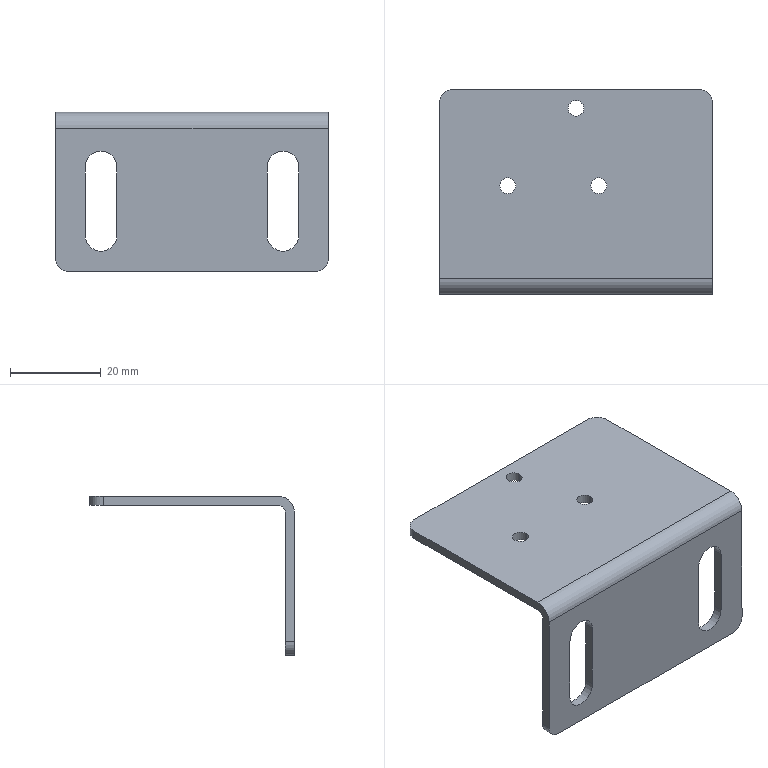Part | SolidWorks | features BaseBody 1 | 1 solid | 30 faces | box 60 x 45 x 35 mm | volume 8584 mm3 | cylinder 18 | plane 12 | commonest cylinder face diameters 7 x7 3.5 x6 6 x4 3 x1
STEP:
#1=CARTESIAN_POINT('',(-16.75,1.35,-2.));
#2=VERTEX_POINT('',#1);
#3=CARTESIAN_POINT('',(-13.25,1.35,-2.));
#4=VERTEX_POINT('',#3);
#5=CARTESIAN_POINT('',(-15.,1.35,-2.));
#6=DIRECTION('',(0.,0.,1.));
#7=DIRECTION('',(1.,0.,0.));
#8=AXIS2_PLACEMENT_3D('',#5,#6,#7);
#9=CIRCLE('',#8,1.75);
#10=EDGE_CURVE('',#2,#4,#9,.T.);
#11=ORIENTED_EDGE('',*,*,#10,.F.);
#12=CARTESIAN_POINT('',(-16.75,1.35,0.));
#13=VERTEX_POINT('',#12);
#14=CARTESIAN_POINT('',(-16.75,1.35,0.));
#15=DIRECTION('',(0.,0.,1.));
#16=VECTOR('',#15,1000.);
#17=LINE('',#14,#16);
#18=EDGE_CURVE('',#2,#13,#17,.T.);
#19=ORIENTED_EDGE('',*,*,#18,.T.);
#20=CARTESIAN_POINT('',(-13.25,1.35,0.));
#21=VERTEX_POINT('',#20);
#22=CARTESIAN_POINT('',(-15.,1.35,0.));
#23=DIRECTION('',(0.,0.,1.));
#24=DIRECTION('',(1.,0.,0.));
#25=AXIS2_PLACEMENT_3D('',#22,#23,#24);
#26=CIRCLE('',#25,1.75);
#27=EDGE_CURVE('',#13,#21,#26,.T.);
#28=ORIENTED_EDGE('',*,*,#27,.T.);
#29=CARTESIAN_POINT('',(-13.25,1.35,0.));
#30=DIRECTION('',(0.,0.,1.));
#31=VECTOR('',#30,1000.);
#32=LINE('',#29,#31);
#33=EDGE_CURVE('',#4,#21,#32,.T.);
#34=ORIENTED_EDGE('',*,*,#33,.F.);
#35=EDGE_LOOP('',(#11,#19,#28,#34));
#36=FACE_OUTER_BOUND('',#35,.T.);
#37=CARTESIAN_POINT('',(-15.,1.35,0.));
#38=DIRECTION('',(0.,0.,1.));
#39=DIRECTION('',(1.,0.,0.));
#40=AXIS2_PLACEMENT_3D('',#37,#38,#39);
#41=CYLINDRICAL_SURFACE('',#40,1.75);
#42=ADVANCED_FACE('',(#36),#41,.F.);
#43=CARTESIAN_POINT('',(3.25,1.35,-2.));
#44=VERTEX_POINT('',#43);
#45=CARTESIAN_POINT('',(6.75,1.35,-2.));
#46=VERTEX_POINT('',#45);
#47=CARTESIAN_POINT('',(5.,1.35,-2.));
#48=DIRECTION('',(0.,0.,1.));
#49=DIRECTION('',(1.,0.,0.));
#50=AXIS2_PLACEMENT_3D('',#47,#48,#49);
#51=CIRCLE('',#50,1.75);
#52=EDGE_CURVE('',#44,#46,#51,.T.);
#53=ORIENTED_EDGE('',*,*,#52,.F.);
#54=CARTESIAN_POINT('',(3.25,1.35,0.));
#55=VERTEX_POINT('',#54);
#56=CARTESIAN_POINT('',(3.25,1.35,0.));
#57=DIRECTION('',(0.,0.,1.));
#58=VECTOR('',#57,1000.);
#59=LINE('',#56,#58);
#60=EDGE_CURVE('',#44,#55,#59,.T.);
#61=ORIENTED_EDGE('',*,*,#60,.T.);
#62=CARTESIAN_POINT('',(6.75,1.35,0.));
#63=VERTEX_POINT('',#62);
#64=CARTESIAN_POINT('',(5.,1.35,0.));
#65=DIRECTION('',(0.,0.,1.));
#66=DIRECTION('',(1.,0.,0.));
#67=AXIS2_PLACEMENT_3D('',#64,#65,#66);
#68=CIRCLE('',#67,1.75);
#69=EDGE_CURVE('',#55,#63,#68,.T.);
#70=ORIENTED_EDGE('',*,*,#69,.T.);
#71=CARTESIAN_POINT('',(6.75,1.35,0.));
#72=DIRECTION('',(0.,0.,1.));
#73=VECTOR('',#72,1000.);
#74=LINE('',#71,#73);
#75=EDGE_CURVE('',#46,#63,#74,.T.);
#76=ORIENTED_EDGE('',*,*,#75,.F.);
#77=EDGE_LOOP('',(#53,#61,#70,#76));
#78=FACE_OUTER_BOUND('',#77,.T.);
#79=CARTESIAN_POINT('',(5.,1.35,0.));
#80=DIRECTION('',(0.,0.,1.));
#81=DIRECTION('',(1.,0.,0.));
#82=AXIS2_PLACEMENT_3D('',#79,#80,#81);
#83=CYLINDRICAL_SURFACE('',#82,1.75);
#84=ADVANCED_FACE('',(#78),#83,.F.);
#85=CARTESIAN_POINT('',(-1.75,18.35,-2.));
#86=VERTEX_POINT('',#85);
#87=CARTESIAN_POINT('',(1.75,18.35,-2.));
#88=VERTEX_POINT('',#87);
#89=CARTESIAN_POINT('',(0.,18.35,-2.));
#90=DIRECTION('',(0.,0.,1.));
#91=DIRECTION('',(1.,0.,0.));
#92=AXIS2_PLACEMENT_3D('',#89,#90,#91);
#93=CIRCLE('',#92,1.75);
#94=EDGE_CURVE('',#86,#88,#93,.T.);
#95=ORIENTED_EDGE('',*,*,#94,.F.);
#96=CARTESIAN_POINT('',(-1.75,18.35,0.));
#97=VERTEX_POINT('',#96);
#98=CARTESIAN_POINT('',(-1.75,18.35,0.));
#99=DIRECTION('',(0.,0.,1.));
#100=VECTOR('',#99,1000.);
#101=LINE('',#98,#100);
#102=EDGE_CURVE('',#86,#97,#101,.T.);
#103=ORIENTED_EDGE('',*,*,#102,.T.);
#104=CARTESIAN_POINT('',(1.75,18.35,0.));
#105=VERTEX_POINT('',#104);
#106=CARTESIAN_POINT('',(0.,18.35,0.));
#107=DIRECTION('',(0.,0.,1.));
#108=DIRECTION('',(1.,0.,0.));
#109=AXIS2_PLACEMENT_3D('',#106,#107,#108);
#110=CIRCLE('',#109,1.75);
#111=EDGE_CURVE('',#97,#105,#110,.T.);
#112=ORIENTED_EDGE('',*,*,#111,.T.);
#113=CARTESIAN_POINT('',(1.75,18.35,0.));
#114=DIRECTION('',(0.,0.,1.));
#115=VECTOR('',#114,1000.);
#116=LINE('',#113,#115);
#117=EDGE_CURVE('',#88,#105,#116,.T.);
#118=ORIENTED_EDGE('',*,*,#117,.F.);
#119=EDGE_LOOP('',(#95,#103,#112,#118));
#120=FACE_OUTER_BOUND('',#119,.T.);
#121=CARTESIAN_POINT('',(0.,18.35,0.));
#122=DIRECTION('',(0.,0.,1.));
#123=DIRECTION('',(1.,0.,0.));
#124=AXIS2_PLACEMENT_3D('',#121,#122,#123);
#125=CYLINDRICAL_SURFACE('',#124,1.75);
#126=ADVANCED_FACE('',(#120),#125,.F.);
#127=CARTESIAN_POINT('',(20.,-22.5,-8.5));
#128=VERTEX_POINT('',#127);
#129=CARTESIAN_POINT('',(23.5,-22.5,-12.));
#130=VERTEX_POINT('',#129);
#131=CARTESIAN_POINT('',(20.,-22.5,-12.));
#132=DIRECTION('',(0.,1.,0.));
#133=DIRECTION('',(0.,0.,1.));
#134=AXIS2_PLACEMENT_3D('',#131,#132,#133);
#135=CIRCLE('',#134,3.5);
#136=EDGE_CURVE('',#128,#130,#135,.T.);
#137=ORIENTED_EDGE('',*,*,#136,.F.);
#138=CARTESIAN_POINT('',(20.,-20.5,-8.5));
#139=VERTEX_POINT('',#138);
#140=CARTESIAN_POINT('',(20.,-30.5,-8.5));
#141=DIRECTION('',(0.,1.,0.));
#142=VECTOR('',#141,1000.);
#143=LINE('',#140,#142);
#144=EDGE_CURVE('',#128,#139,#143,.T.);
#145=ORIENTED_EDGE('',*,*,#144,.T.);
#146=CARTESIAN_POINT('',(23.5,-20.5,-12.));
#147=VERTEX_POINT('',#146);
#148=CARTESIAN_POINT('',(20.,-20.5,-12.));
#149=DIRECTION('',(0.,-1.,0.));
#150=DIRECTION('',(0.,0.,1.));
#151=AXIS2_PLACEMENT_3D('',#148,#149,#150);
#152=CIRCLE('',#151,3.5);
#153=EDGE_CURVE('',#147,#139,#152,.T.);
#154=ORIENTED_EDGE('',*,*,#153,.F.);
#155=CARTESIAN_POINT('',(23.5,-30.5,-12.));
#156=DIRECTION('',(0.,-1.,0.));
#157=VECTOR('',#156,1000.);
#158=LINE('',#155,#157);
#159=EDGE_CURVE('',#147,#130,#158,.T.);
#160=ORIENTED_EDGE('',*,*,#159,.T.);
#161=EDGE_LOOP('',(#137,#145,#154,#160));
#162=FACE_OUTER_BOUND('',#161,.T.);
#163=CARTESIAN_POINT('',(20.,-30.5,-12.));
#164=DIRECTION('',(0.,1.,0.));
#165=DIRECTION('',(0.,0.,1.));
#166=AXIS2_PLACEMENT_3D('',#163,#164,#165);
#167=CYLINDRICAL_SURFACE('',#166,3.5);
#168=ADVANCED_FACE('',(#162),#167,.F.);
#169=CARTESIAN_POINT('',(-20.,-22.5,-8.5));
#170=VERTEX_POINT('',#169);
#171=CARTESIAN_POINT('',(-16.5,-22.5,-12.));
#172=VERTEX_POINT('',#171);
#173=CARTESIAN_POINT('',(-20.,-22.5,-12.));
#174=DIRECTION('',(0.,1.,0.));
#175=DIRECTION('',(0.,0.,1.));
#176=AXIS2_PLACEMENT_3D('',#173,#174,#175);
#177=CIRCLE('',#176,3.5);
#178=EDGE_CURVE('',#170,#172,#177,.T.);
#179=ORIENTED_EDGE('',*,*,#178,.F.);
#180=CARTESIAN_POINT('',(-20.,-20.5,-8.5));
#181=VERTEX_POINT('',#180);
#182=CARTESIAN_POINT('',(-20.,-30.5,-8.5));
#183=DIRECTION('',(0.,1.,0.));
#184=VECTOR('',#183,1000.);
#185=LINE('',#182,#184);
#186=EDGE_CURVE('',#170,#181,#185,.T.);
#187=ORIENTED_EDGE('',*,*,#186,.T.);
#188=CARTESIAN_POINT('',(-16.5,-20.5,-12.));
#189=VERTEX_POINT('',#188);
#190=CARTESIAN_POINT('',(-20.,-20.5,-12.));
#191=DIRECTION('',(0.,-1.,0.));
#192=DIRECTION('',(0.,0.,1.));
#193=AXIS2_PLACEMENT_3D('',#190,#191,#192);
#194=CIRCLE('',#193,3.5);
#195=EDGE_CURVE('',#189,#181,#194,.T.);
#196=ORIENTED_EDGE('',*,*,#195,.F.);
#197=CARTESIAN_POINT('',(-16.5,-30.5,-12.));
#198=DIRECTION('',(0.,-1.,0.));
#199=VECTOR('',#198,1000.);
#200=LINE('',#197,#199);
#201=EDGE_CURVE('',#189,#172,#200,.T.);
#202=ORIENTED_EDGE('',*,*,#201,.T.);
#203=EDGE_LOOP('',(#179,#187,#196,#202));
#204=FACE_OUTER_BOUND('',#203,.T.);
#205=CARTESIAN_POINT('',(-20.,-30.5,-12.));
#206=DIRECTION('',(0.,1.,0.));
#207=DIRECTION('',(0.,0.,1.));
#208=AXIS2_PLACEMENT_3D('',#205,#206,#207);
#209=CYLINDRICAL_SURFACE('',#208,3.5);
#210=ADVANCED_FACE('',(#204),#209,.F.);
#211=CARTESIAN_POINT('',(-30.,19.5,0.));
#212=VERTEX_POINT('',#211);
#213=CARTESIAN_POINT('',(-27.,22.5,0.));
#214=VERTEX_POINT('',#213);
#215=CARTESIAN_POINT('',(-27.,19.5,0.));
#216=DIRECTION('',(0.,0.,-1.));
#217=DIRECTION('',(1.,0.,0.));
#218=AXIS2_PLACEMENT_3D('',#215,#216,#217);
#219=CIRCLE('',#218,3.);
#220=EDGE_CURVE('',#212,#214,#219,.T.);
#221=ORIENTED_EDGE('',*,*,#220,.F.);
#222=CARTESIAN_POINT('',(-30.,-19.,0.));
#223=VERTEX_POINT('',#222);
#224=CARTESIAN_POINT('',(-30.,0.,0.));
#225=DIRECTION('',(0.,1.,0.));
#226=VECTOR('',#225,1000.);
#227=LINE('',#224,#226);
#228=EDGE_CURVE('',#223,#212,#227,.T.);
#229=ORIENTED_EDGE('',*,*,#228,.F.);
#230=CARTESIAN_POINT('',(30.,-19.,0.));
#231=VERTEX_POINT('',#230);
#232=CARTESIAN_POINT('',(0.,-19.,0.));
#233=DIRECTION('',(-1.,0.,0.));
#234=VECTOR('',#233,1000.);
#235=LINE('',#232,#234);
#236=EDGE_CURVE('',#231,#223,#235,.T.);
#237=ORIENTED_EDGE('',*,*,#236,.F.);
#238=CARTESIAN_POINT('',(30.,19.5,0.));
#239=VERTEX_POINT('',#238);
#240=CARTESIAN_POINT('',(30.,0.,0.));
#241=DIRECTION('',(0.,-1.,0.));
#242=VECTOR('',#241,1000.);
#243=LINE('',#240,#242);
#244=EDGE_CURVE('',#239,#231,#243,.T.);
#245=ORIENTED_EDGE('',*,*,#244,.F.);
#246=CARTESIAN_POINT('',(27.,22.5,0.));
#247=VERTEX_POINT('',#246);
#248=CARTESIAN_POINT('',(27.,19.5,0.));
#249=DIRECTION('',(0.,0.,-1.));
#250=DIRECTION('',(1.,0.,0.));
#251=AXIS2_PLACEMENT_3D('',#248,#249,#250);
#252=CIRCLE('',#251,3.);
#253=EDGE_CURVE('',#247,#239,#252,.T.);
#254=ORIENTED_EDGE('',*,*,#253,.F.);
#255=CARTESIAN_POINT('',(0.,22.5,0.));
#256=DIRECTION('',(1.,0.,0.));
#257=VECTOR('',#256,1000.);
#258=LINE('',#255,#257);
#259=EDGE_CURVE('',#214,#247,#258,.T.);
#260=ORIENTED_EDGE('',*,*,#259,.F.);
#261=EDGE_LOOP('',(#221,#229,#237,#245,#254,#260));
#262=FACE_OUTER_BOUND('',#261,.T.);
#263=CARTESIAN_POINT('',(-15.,1.35,0.));
#264=DIRECTION('',(0.,0.,1.));
#265=DIRECTION('',(1.,0.,0.));
#266=AXIS2_PLACEMENT_3D('',#263,#264,#265);
#267=CIRCLE('',#266,1.75);
#268=EDGE_CURVE('',#21,#13,#267,.T.);
#269=ORIENTED_EDGE('',*,*,#268,.F.);
#270=ORIENTED_EDGE('',*,*,#27,.F.);
#271=EDGE_LOOP('',(#269,#270));
#272=FACE_BOUND('',#271,.T.);
#273=CARTESIAN_POINT('',(5.,1.35,0.));
#274=DIRECTION('',(0.,0.,1.));
#275=DIRECTION('',(1.,0.,0.));
#276=AXIS2_PLACEMENT_3D('',#273,#274,#275);
#277=CIRCLE('',#276,1.75);
#278=EDGE_CURVE('',#63,#55,#277,.T.);
#279=ORIENTED_EDGE('',*,*,#278,.F.);
#280=ORIENTED_EDGE('',*,*,#69,.F.);
#281=EDGE_LOOP('',(#279,#280));
#282=FACE_BOUND('',#281,.T.);
#283=CARTESIAN_POINT('',(0.,18.35,0.));
#284=DIRECTION('',(0.,0.,1.));
#285=DIRECTION('',(1.,0.,0.));
#286=AXIS2_PLACEMENT_3D('',#283,#284,#285);
#287=CIRCLE('',#286,1.75);
#288=EDGE_CURVE('',#105,#97,#287,.T.);
#289=ORIENTED_EDGE('',*,*,#288,.F.);
#290=ORIENTED_EDGE('',*,*,#111,.F.);
#291=EDGE_LOOP('',(#289,#290));
#292=FACE_BOUND('',#291,.T.);
#293=CARTESIAN_POINT('',(0.,0.,0.));
#294=DIRECTION('',(0.,0.,-1.));
#295=DIRECTION('',(-1.,0.,0.));
#296=AXIS2_PLACEMENT_3D('',#293,#294,#295);
#297=PLANE('',#296);
#298=ADVANCED_FACE('',(#262,#272,#282,#292),#297,.F.);
#299=ORIENTED_EDGE('',*,*,#259,.T.);
#300=CARTESIAN_POINT('',(27.,22.5,-2.));
#301=VERTEX_POINT('',#300);
#302=CARTESIAN_POINT('',(27.,22.5,-2.));
#303=DIRECTION('',(0.,0.,-1.));
#304=VECTOR('',#303,1000.);
#305=LINE('',#302,#304);
#306=EDGE_CURVE('',#247,#301,#305,.T.);
#307=ORIENTED_EDGE('',*,*,#306,.T.);
#308=CARTESIAN_POINT('',(-27.,22.5,-2.));
#309=VERTEX_POINT('',#308);
#310=CARTESIAN_POINT('',(-30.,22.5,-2.));
#311=DIRECTION('',(-1.,0.,0.));
#312=VECTOR('',#311,1000.);
#313=LINE('',#310,#312);
#314=EDGE_CURVE('',#301,#309,#313,.T.);
#315=ORIENTED_EDGE('',*,*,#314,.T.);
#316=CARTESIAN_POINT('',(-27.,22.5,-2.));
#317=DIRECTION('',(0.,0.,1.));
#318=VECTOR('',#317,1000.);
#319=LINE('',#316,#318);
#320=EDGE_CURVE('',#309,#214,#319,.T.);
#321=ORIENTED_EDGE('',*,*,#320,.T.);
#322=EDGE_LOOP('',(#299,#307,#315,#321));
#323=FACE_OUTER_BOUND('',#322,.T.);
#324=CARTESIAN_POINT('',(-30.,22.5,-2.));
#325=DIRECTION('',(0.,1.,0.));
#326=DIRECTION('',(0.,0.,1.));
#327=AXIS2_PLACEMENT_3D('',#324,#325,#326);
#328=PLANE('',#327);
#329=ADVANCED_FACE('',(#323),#328,.T.);
#330=ORIENTED_EDGE('',*,*,#220,.T.);
#331=ORIENTED_EDGE('',*,*,#320,.F.);
#332=CARTESIAN_POINT('',(-30.,19.5,-2.));
#333=VERTEX_POINT('',#332);
#334=CARTESIAN_POINT('',(-27.,19.5,-2.));
#335=DIRECTION('',(0.,0.,1.));
#336=DIRECTION('',(1.,0.,0.));
#337=AXIS2_PLACEMENT_3D('',#334,#335,#336);
#338=CIRCLE('',#337,3.);
#339=EDGE_CURVE('',#309,#333,#338,.T.);
#340=ORIENTED_EDGE('',*,*,#339,.T.);
#341=CARTESIAN_POINT('',(-30.,19.5,-2.));
#342=DIRECTION('',(0.,0.,1.));
#343=VECTOR('',#342,1000.);
#344=LINE('',#341,#343);
#345=EDGE_CURVE('',#333,#212,#344,.T.);
#346=ORIENTED_EDGE('',*,*,#345,.T.);
#347=EDGE_LOOP('',(#330,#331,#340,#346));
#348=FACE_OUTER_BOUND('',#347,.T.);
#349=CARTESIAN_POINT('',(-27.,19.5,-2.));
#350=DIRECTION('',(0.,0.,1.));
#351=DIRECTION('',(1.,0.,0.));
#352=AXIS2_PLACEMENT_3D('',#349,#350,#351);
#353=CYLINDRICAL_SURFACE('',#352,3.);
#354=ADVANCED_FACE('',(#348),#353,.T.);
#355=CARTESIAN_POINT('',(-30.,-19.,-2.));
#356=VERTEX_POINT('',#355);
#357=CARTESIAN_POINT('',(-30.,-22.5,-2.));
#358=DIRECTION('',(0.,-1.,0.));
#359=VECTOR('',#358,1000.);
#360=LINE('',#357,#359);
#361=EDGE_CURVE('',#333,#356,#360,.T.);
#362=ORIENTED_EDGE('',*,*,#361,.T.);
#363=CARTESIAN_POINT('',(-30.,-20.5,-3.5));
#364=VERTEX_POINT('',#363);
#365=CARTESIAN_POINT('',(-30.,-19.,-3.5));
#366=DIRECTION('',(-1.,0.,0.));
#367=DIRECTION('',(0.,0.,1.));
#368=AXIS2_PLACEMENT_3D('',#365,#366,#367);
#369=CIRCLE('',#368,1.5);
#370=EDGE_CURVE('',#364,#356,#369,.T.);
#371=ORIENTED_EDGE('',*,*,#370,.F.);
#372=CARTESIAN_POINT('',(-30.,-20.5,-32.));
#373=VERTEX_POINT('',#372);
#374=CARTESIAN_POINT('',(-30.,-20.5,-2.));
#375=DIRECTION('',(0.,0.,-1.));
#376=VECTOR('',#375,1000.);
#377=LINE('',#374,#376);
#378=EDGE_CURVE('',#364,#373,#377,.T.);
#379=ORIENTED_EDGE('',*,*,#378,.T.);
#380=CARTESIAN_POINT('',(-30.,-22.5,-32.));
#381=VERTEX_POINT('',#380);
#382=CARTESIAN_POINT('',(-30.,-22.5,-32.));
#383=DIRECTION('',(0.,-1.,0.));
#384=VECTOR('',#383,1000.);
#385=LINE('',#382,#384);
#386=EDGE_CURVE('',#373,#381,#385,.T.);
#387=ORIENTED_EDGE('',*,*,#386,.T.);
#388=CARTESIAN_POINT('',(-30.,-22.5,-3.5));
#389=VERTEX_POINT('',#388);
#390=CARTESIAN_POINT('',(-30.,-22.5,0.));
#391=DIRECTION('',(0.,0.,-1.));
#392=VECTOR('',#391,1000.);
#393=LINE('',#390,#392);
#394=EDGE_CURVE('',#389,#381,#393,.T.);
#395=ORIENTED_EDGE('',*,*,#394,.F.);
#396=CARTESIAN_POINT('',(-30.,-19.,-3.5));
#397=DIRECTION('',(1.,0.,0.));
#398=DIRECTION('',(0.,0.,1.));
#399=AXIS2_PLACEMENT_3D('',#396,#397,#398);
#400=CIRCLE('',#399,3.5);
#401=EDGE_CURVE('',#223,#389,#400,.T.);
#402=ORIENTED_EDGE('',*,*,#401,.F.);
#403=ORIENTED_EDGE('',*,*,#228,.T.);
#404=ORIENTED_EDGE('',*,*,#345,.F.);
#405=EDGE_LOOP('',(#362,#371,#379,#387,#395,#402,#403,#404));
#406=FACE_OUTER_BOUND('',#405,.T.);
#407=CARTESIAN_POINT('',(-30.,-22.5,-2.));
#408=DIRECTION('',(-1.,0.,0.));
#409=DIRECTION('',(0.,0.,1.));
#410=AXIS2_PLACEMENT_3D('',#407,#408,#409);
#411=PLANE('',#410);
#412=ADVANCED_FACE('',(#406),#411,.T.);
#413=CARTESIAN_POINT('',(30.,-22.5,-3.5));
#414=VERTEX_POINT('',#413);
#415=CARTESIAN_POINT('',(-30.,-22.5,-3.5));
#416=DIRECTION('',(1.,0.,0.));
#417=VECTOR('',#416,1000.);
#418=LINE('',#415,#417);
#419=EDGE_CURVE('',#389,#414,#418,.T.);
#420=ORIENTED_EDGE('',*,*,#419,.T.);
#421=CARTESIAN_POINT('',(30.,-19.,-3.5));
#422=DIRECTION('',(-1.,0.,0.));
#423=DIRECTION('',(0.,0.,1.));
#424=AXIS2_PLACEMENT_3D('',#421,#422,#423);
#425=CIRCLE('',#424,3.5);
#426=EDGE_CURVE('',#414,#231,#425,.T.);
#427=ORIENTED_EDGE('',*,*,#426,.T.);
#428=ORIENTED_EDGE('',*,*,#236,.T.);
#429=ORIENTED_EDGE('',*,*,#401,.T.);
#430=EDGE_LOOP('',(#420,#427,#428,#429));
#431=FACE_OUTER_BOUND('',#430,.T.);
#432=CARTESIAN_POINT('',(-30.,-19.,-3.5));
#433=DIRECTION('',(-1.,0.,0.));
#434=DIRECTION('',(0.,0.,1.));
#435=AXIS2_PLACEMENT_3D('',#432,#433,#434);
#436=CYLINDRICAL_SURFACE('',#435,3.5);
#437=ADVANCED_FACE('',(#431),#436,.T.);
#438=ORIENTED_EDGE('',*,*,#244,.T.);
#439=ORIENTED_EDGE('',*,*,#426,.F.);
#440=CARTESIAN_POINT('',(30.,-22.5,-32.));
#441=VERTEX_POINT('',#440);
#442=CARTESIAN_POINT('',(30.,-22.5,0.));
#443=DIRECTION('',(0.,0.,1.));
#444=VECTOR('',#443,1000.);
#445=LINE('',#442,#444);
#446=EDGE_CURVE('',#441,#414,#445,.T.);
#447=ORIENTED_EDGE('',*,*,#446,.F.);
#448=CARTESIAN_POINT('',(30.,-20.5,-32.));
#449=VERTEX_POINT('',#448);
#450=CARTESIAN_POINT('',(30.,-22.5,-32.));
#451=DIRECTION('',(0.,1.,0.));
#452=VECTOR('',#451,1000.);
#453=LINE('',#450,#452);
#454=EDGE_CURVE('',#441,#449,#453,.T.);
#455=ORIENTED_EDGE('',*,*,#454,.T.);
#456=CARTESIAN_POINT('',(30.,-20.5,-3.5));
#457=VERTEX_POINT('',#456);
#458=CARTESIAN_POINT('',(30.,-20.5,-35.));
#459=DIRECTION('',(0.,0.,1.));
#460=VECTOR('',#459,1000.);
#461=LINE('',#458,#460);
#462=EDGE_CURVE('',#449,#457,#461,.T.);
#463=ORIENTED_EDGE('',*,*,#462,.T.);
#464=CARTESIAN_POINT('',(30.,-19.,-2.));
#465=VERTEX_POINT('',#464);
#466=CARTESIAN_POINT('',(30.,-19.,-3.5));
#467=DIRECTION('',(-1.,0.,0.));
#468=DIRECTION('',(0.,0.,1.));
#469=AXIS2_PLACEMENT_3D('',#466,#467,#468);
#470=CIRCLE('',#469,1.5);
#471=EDGE_CURVE('',#457,#465,#470,.T.);
#472=ORIENTED_EDGE('',*,*,#471,.T.);
#473=CARTESIAN_POINT('',(30.,19.5,-2.));
#474=VERTEX_POINT('',#473);
#475=CARTESIAN_POINT('',(30.,-22.5,-2.));
#476=DIRECTION('',(0.,1.,0.));
#477=VECTOR('',#476,1000.);
#478=LINE('',#475,#477);
#479=EDGE_CURVE('',#465,#474,#478,.T.);
#480=ORIENTED_EDGE('',*,*,#479,.T.);
#481=CARTESIAN_POINT('',(30.,19.5,-2.));
#482=DIRECTION('',(0.,0.,1.));
#483=VECTOR('',#482,1000.);
#484=LINE('',#481,#483);
#485=EDGE_CURVE('',#474,#239,#484,.T.);
#486=ORIENTED_EDGE('',*,*,#485,.T.);
#487=EDGE_LOOP('',(#438,#439,#447,#455,#463,#472,#480,#486));
#488=FACE_OUTER_BOUND('',#487,.T.);
#489=CARTESIAN_POINT('',(30.,-22.5,-2.));
#490=DIRECTION('',(1.,0.,0.));
#491=DIRECTION('',(0.,0.,-1.));
#492=AXIS2_PLACEMENT_3D('',#489,#490,#491);
#493=PLANE('',#492);
#494=ADVANCED_FACE('',(#488),#493,.T.);
#495=ORIENTED_EDGE('',*,*,#253,.T.);
#496=ORIENTED_EDGE('',*,*,#485,.F.);
#497=CARTESIAN_POINT('',(27.,19.5,-2.));
#498=DIRECTION('',(0.,0.,1.));
#499=DIRECTION('',(1.,0.,0.));
#500=AXIS2_PLACEMENT_3D('',#497,#498,#499);
#501=CIRCLE('',#500,3.);
#502=EDGE_CURVE('',#474,#301,#501,.T.);
#503=ORIENTED_EDGE('',*,*,#502,.T.);
#504=ORIENTED_EDGE('',*,*,#306,.F.);
#505=EDGE_LOOP('',(#495,#496,#503,#504));
#506=FACE_OUTER_BOUND('',#505,.T.);
#507=CARTESIAN_POINT('',(27.,19.5,-2.));
#508=DIRECTION('',(0.,0.,1.));
#509=DIRECTION('',(1.,0.,0.));
#510=AXIS2_PLACEMENT_3D('',#507,#508,#509);
#511=CYLINDRICAL_SURFACE('',#510,3.);
#512=ADVANCED_FACE('',(#506),#511,.T.);
#513=ORIENTED_EDGE('',*,*,#18,.F.);
#514=CARTESIAN_POINT('',(-15.,1.35,-2.));
#515=DIRECTION('',(0.,0.,1.));
#516=DIRECTION('',(1.,0.,0.));
#517=AXIS2_PLACEMENT_3D('',#514,#515,#516);
#518=CIRCLE('',#517,1.75);
#519=EDGE_CURVE('',#4,#2,#518,.T.);
#520=ORIENTED_EDGE('',*,*,#519,.F.);
#521=ORIENTED_EDGE('',*,*,#33,.T.);
#522=ORIENTED_EDGE('',*,*,#268,.T.);
#523=EDGE_LOOP('',(#513,#520,#521,#522));
#524=FACE_OUTER_BOUND('',#523,.T.);
#525=CARTESIAN_POINT('',(-15.,1.35,0.));
#526=DIRECTION('',(0.,0.,1.));
#527=DIRECTION('',(1.,0.,0.));
#528=AXIS2_PLACEMENT_3D('',#525,#526,#527);
#529=CYLINDRICAL_SURFACE('',#528,1.75);
#530=ADVANCED_FACE('',(#524),#529,.F.);
#531=ORIENTED_EDGE('',*,*,#60,.F.);
#532=CARTESIAN_POINT('',(5.,1.35,-2.));
#533=DIRECTION('',(0.,0.,1.));
#534=DIRECTION('',(1.,0.,0.));
#535=AXIS2_PLACEMENT_3D('',#532,#533,#534);
#536=CIRCLE('',#535,1.75);
#537=EDGE_CURVE('',#46,#44,#536,.T.);
#538=ORIENTED_EDGE('',*,*,#537,.F.);
#539=ORIENTED_EDGE('',*,*,#75,.T.);
#540=ORIENTED_EDGE('',*,*,#278,.T.);
#541=EDGE_LOOP('',(#531,#538,#539,#540));
#542=FACE_OUTER_BOUND('',#541,.T.);
#543=CARTESIAN_POINT('',(5.,1.35,0.));
#544=DIRECTION('',(0.,0.,1.));
#545=DIRECTION('',(1.,0.,0.));
#546=AXIS2_PLACEMENT_3D('',#543,#544,#545);
#547=CYLINDRICAL_SURFACE('',#546,1.75);
#548=ADVANCED_FACE('',(#542),#547,.F.);
#549=ORIENTED_EDGE('',*,*,#102,.F.);
#550=CARTESIAN_POINT('',(0.,18.35,-2.));
#551=DIRECTION('',(0.,0.,1.));
#552=DIRECTION('',(1.,0.,0.));
#553=AXIS2_PLACEMENT_3D('',#550,#551,#552);
#554=CIRCLE('',#553,1.75);
#555=EDGE_CURVE('',#88,#86,#554,.T.);
#556=ORIENTED_EDGE('',*,*,#555,.F.);
#557=ORIENTED_EDGE('',*,*,#117,.T.);
#558=ORIENTED_EDGE('',*,*,#288,.T.);
#559=EDGE_LOOP('',(#549,#556,#557,#558));
#560=FACE_OUTER_BOUND('',#559,.T.);
#561=CARTESIAN_POINT('',(0.,18.35,0.));
#562=DIRECTION('',(0.,0.,1.));
#563=DIRECTION('',(1.,0.,0.));
#564=AXIS2_PLACEMENT_3D('',#561,#562,#563);
#565=CYLINDRICAL_SURFACE('',#564,1.75);
#566=ADVANCED_FACE('',(#560),#565,.F.);
#567=ORIENTED_EDGE('',*,*,#479,.F.);
#568=CARTESIAN_POINT('',(0.,-19.,-2.));
#569=DIRECTION('',(-1.,0.,0.));
#570=VECTOR('',#569,1000.);
#571=LINE('',#568,#570);
#572=EDGE_CURVE('',#465,#356,#571,.T.);
#573=ORIENTED_EDGE('',*,*,#572,.T.);
#574=ORIENTED_EDGE('',*,*,#361,.F.);
#575=ORIENTED_EDGE('',*,*,#339,.F.);
#576=ORIENTED_EDGE('',*,*,#314,.F.);
#577=ORIENTED_EDGE('',*,*,#502,.F.);
#578=EDGE_LOOP('',(#567,#573,#574,#575,#576,#577));
#579=FACE_OUTER_BOUND('',#578,.T.);
#580=ORIENTED_EDGE('',*,*,#519,.T.);
#581=ORIENTED_EDGE('',*,*,#10,.T.);
#582=EDGE_LOOP('',(#580,#581));
#583=FACE_BOUND('',#582,.T.);
#584=ORIENTED_EDGE('',*,*,#537,.T.);
#585=ORIENTED_EDGE('',*,*,#52,.T.);
#586=EDGE_LOOP('',(#584,#585));
#587=FACE_BOUND('',#586,.T.);
#588=ORIENTED_EDGE('',*,*,#555,.T.);
#589=ORIENTED_EDGE('',*,*,#94,.T.);
#590=EDGE_LOOP('',(#588,#589));
#591=FACE_BOUND('',#590,.T.);
#592=CARTESIAN_POINT('',(0.,0.,-2.));
#593=DIRECTION('',(0.,0.,-1.));
#594=DIRECTION('',(-1.,0.,0.));
#595=AXIS2_PLACEMENT_3D('',#592,#593,#594);
#596=PLANE('',#595);
#597=ADVANCED_FACE('',(#579,#583,#587,#591),#596,.T.);
#598=ORIENTED_EDGE('',*,*,#394,.T.);
#599=CARTESIAN_POINT('',(-27.,-22.5,-35.));
#600=VERTEX_POINT('',#599);
#601=CARTESIAN_POINT('',(-27.,-22.5,-32.));
#602=DIRECTION('',(0.,-1.,0.));
#603=DIRECTION('',(0.,0.,1.));
#604=AXIS2_PLACEMENT_3D('',#601,#602,#603);
#605=CIRCLE('',#604,3.);
#606=EDGE_CURVE('',#381,#600,#605,.T.);
#607=ORIENTED_EDGE('',*,*,#606,.T.);
#608=CARTESIAN_POINT('',(27.,-22.5,-35.));
#609=VERTEX_POINT('',#608);
#610=CARTESIAN_POINT('',(0.,-22.5,-35.));
#611=DIRECTION('',(1.,0.,0.));
#612=VECTOR('',#611,1000.);
#613=LINE('',#610,#612);
#614=EDGE_CURVE('',#600,#609,#613,.T.);
#615=ORIENTED_EDGE('',*,*,#614,.T.);
#616=CARTESIAN_POINT('',(27.,-22.5,-32.));
#617=DIRECTION('',(0.,-1.,0.));
#618=DIRECTION('',(0.,0.,1.));
#619=AXIS2_PLACEMENT_3D('',#616,#617,#618);
#620=CIRCLE('',#619,3.);
#621=EDGE_CURVE('',#609,#441,#620,.T.);
#622=ORIENTED_EDGE('',*,*,#621,.T.);
#623=ORIENTED_EDGE('',*,*,#446,.T.);
#624=ORIENTED_EDGE('',*,*,#419,.F.);
#625=EDGE_LOOP('',(#598,#607,#615,#622,#623,#624));
#626=FACE_OUTER_BOUND('',#625,.T.);
#627=CARTESIAN_POINT('',(16.5,-22.5,-27.));
#628=VERTEX_POINT('',#627);
#629=CARTESIAN_POINT('',(16.5,-22.5,-12.));
#630=VERTEX_POINT('',#629);
#631=CARTESIAN_POINT('',(16.5,-22.5,0.));
#632=DIRECTION('',(0.,0.,1.));
#633=VECTOR('',#632,1000.);
#634=LINE('',#631,#633);
#635=EDGE_CURVE('',#628,#630,#634,.T.);
#636=ORIENTED_EDGE('',*,*,#635,.T.);
#637=CARTESIAN_POINT('',(20.,-22.5,-12.));
#638=DIRECTION('',(0.,1.,0.));
#639=DIRECTION('',(0.,0.,1.));
#640=AXIS2_PLACEMENT_3D('',#637,#638,#639);
#641=CIRCLE('',#640,3.5);
#642=EDGE_CURVE('',#630,#128,#641,.T.);
#643=ORIENTED_EDGE('',*,*,#642,.T.);
#644=ORIENTED_EDGE('',*,*,#136,.T.);
#645=CARTESIAN_POINT('',(23.5,-22.5,-27.));
#646=VERTEX_POINT('',#645);
#647=CARTESIAN_POINT('',(23.5,-22.5,0.));
#648=DIRECTION('',(0.,0.,-1.));
#649=VECTOR('',#648,1000.);
#650=LINE('',#647,#649);
#651=EDGE_CURVE('',#130,#646,#650,.T.);
#652=ORIENTED_EDGE('',*,*,#651,.T.);
#653=CARTESIAN_POINT('',(20.,-22.5,-27.));
#654=DIRECTION('',(0.,1.,0.));
#655=DIRECTION('',(0.,0.,1.));
#656=AXIS2_PLACEMENT_3D('',#653,#654,#655);
#657=CIRCLE('',#656,3.5);
#658=EDGE_CURVE('',#646,#628,#657,.T.);
#659=ORIENTED_EDGE('',*,*,#658,.T.);
#660=EDGE_LOOP('',(#636,#643,#644,#652,#659));
#661=FACE_BOUND('',#660,.T.);
#662=CARTESIAN_POINT('',(-23.5,-22.5,-27.));
#663=VERTEX_POINT('',#662);
#664=CARTESIAN_POINT('',(-23.5,-22.5,-12.));
#665=VERTEX_POINT('',#664);
#666=CARTESIAN_POINT('',(-23.5,-22.5,0.));
#667=DIRECTION('',(0.,0.,1.));
#668=VECTOR('',#667,1000.);
#669=LINE('',#666,#668);
#670=EDGE_CURVE('',#663,#665,#669,.T.);
#671=ORIENTED_EDGE('',*,*,#670,.T.);
#672=CARTESIAN_POINT('',(-20.,-22.5,-12.));
#673=DIRECTION('',(0.,1.,0.));
#674=DIRECTION('',(0.,0.,1.));
#675=AXIS2_PLACEMENT_3D('',#672,#673,#674);
#676=CIRCLE('',#675,3.5);
#677=EDGE_CURVE('',#665,#170,#676,.T.);
#678=ORIENTED_EDGE('',*,*,#677,.T.);
#679=ORIENTED_EDGE('',*,*,#178,.T.);
#680=CARTESIAN_POINT('',(-16.5,-22.5,-27.));
#681=VERTEX_POINT('',#680);
#682=CARTESIAN_POINT('',(-16.5,-22.5,0.));
#683=DIRECTION('',(0.,0.,-1.));
#684=VECTOR('',#683,1000.);
#685=LINE('',#682,#684);
#686=EDGE_CURVE('',#172,#681,#685,.T.);
#687=ORIENTED_EDGE('',*,*,#686,.T.);
#688=CARTESIAN_POINT('',(-20.,-22.5,-27.));
#689=DIRECTION('',(0.,1.,0.));
#690=DIRECTION('',(0.,0.,1.));
#691=AXIS2_PLACEMENT_3D('',#688,#689,#690);
#692=CIRCLE('',#691,3.5);
#693=EDGE_CURVE('',#681,#663,#692,.T.);
#694=ORIENTED_EDGE('',*,*,#693,.T.);
#695=EDGE_LOOP('',(#671,#678,#679,#687,#694));
#696=FACE_BOUND('',#695,.T.);
#697=CARTESIAN_POINT('',(0.,-22.5,0.));
#698=DIRECTION('',(0.,-1.,0.));
#699=DIRECTION('',(0.,0.,-1.));
#700=AXIS2_PLACEMENT_3D('',#697,#698,#699);
#701=PLANE('',#700);
#702=ADVANCED_FACE('',(#626,#661,#696),#701,.T.);
#703=ORIENTED_EDGE('',*,*,#471,.F.);
#704=CARTESIAN_POINT('',(-30.,-20.5,-3.5));
#705=DIRECTION('',(1.,0.,0.));
#706=VECTOR('',#705,1000.);
#707=LINE('',#704,#706);
#708=EDGE_CURVE('',#364,#457,#707,.T.);
#709=ORIENTED_EDGE('',*,*,#708,.F.);
#710=ORIENTED_EDGE('',*,*,#370,.T.);
#711=ORIENTED_EDGE('',*,*,#572,.F.);
#712=EDGE_LOOP('',(#703,#709,#710,#711));
#713=FACE_OUTER_BOUND('',#712,.T.);
#714=CARTESIAN_POINT('',(-30.,-19.,-3.5));
#715=DIRECTION('',(-1.,0.,0.));
#716=DIRECTION('',(0.,0.,1.));
#717=AXIS2_PLACEMENT_3D('',#714,#715,#716);
#718=CYLINDRICAL_SURFACE('',#717,1.5);
#719=ADVANCED_FACE('',(#713),#718,.F.);
#720=CARTESIAN_POINT('',(-27.,-20.5,-35.));
#721=VERTEX_POINT('',#720);
#722=CARTESIAN_POINT('',(-27.,-20.5,-32.));
#723=DIRECTION('',(0.,-1.,0.));
#724=DIRECTION('',(0.,0.,1.));
#725=AXIS2_PLACEMENT_3D('',#722,#723,#724);
#726=CIRCLE('',#725,3.);
#727=EDGE_CURVE('',#373,#721,#726,.T.);
#728=ORIENTED_EDGE('',*,*,#727,.T.);
#729=CARTESIAN_POINT('',(-27.,-22.5,-35.));
#730=DIRECTION('',(0.,-1.,0.));
#731=VECTOR('',#730,1000.);
#732=LINE('',#729,#731);
#733=EDGE_CURVE('',#721,#600,#732,.T.);
#734=ORIENTED_EDGE('',*,*,#733,.T.);
#735=ORIENTED_EDGE('',*,*,#606,.F.);
#736=ORIENTED_EDGE('',*,*,#386,.F.);
#737=EDGE_LOOP('',(#728,#734,#735,#736));
#738=FACE_OUTER_BOUND('',#737,.T.);
#739=CARTESIAN_POINT('',(-27.,-22.5,-32.));
#740=DIRECTION('',(0.,1.,0.));
#741=DIRECTION('',(0.,0.,1.));
#742=AXIS2_PLACEMENT_3D('',#739,#740,#741);
#743=CYLINDRICAL_SURFACE('',#742,3.);
#744=ADVANCED_FACE('',(#738),#743,.T.);
#745=CARTESIAN_POINT('',(27.,-20.5,-35.));
#746=VERTEX_POINT('',#745);
#747=CARTESIAN_POINT('',(27.,-20.5,-32.));
#748=DIRECTION('',(0.,-1.,0.));
#749=DIRECTION('',(0.,0.,1.));
#750=AXIS2_PLACEMENT_3D('',#747,#748,#749);
#751=CIRCLE('',#750,3.);
#752=EDGE_CURVE('',#746,#449,#751,.T.);
#753=ORIENTED_EDGE('',*,*,#752,.T.);
#754=ORIENTED_EDGE('',*,*,#454,.F.);
#755=ORIENTED_EDGE('',*,*,#621,.F.);
#756=CARTESIAN_POINT('',(27.,-22.5,-35.));
#757=DIRECTION('',(0.,1.,0.));
#758=VECTOR('',#757,1000.);
#759=LINE('',#756,#758);
#760=EDGE_CURVE('',#609,#746,#759,.T.);
#761=ORIENTED_EDGE('',*,*,#760,.T.);
#762=EDGE_LOOP('',(#753,#754,#755,#761));
#763=FACE_OUTER_BOUND('',#762,.T.);
#764=CARTESIAN_POINT('',(27.,-22.5,-32.));
#765=DIRECTION('',(0.,1.,0.));
#766=DIRECTION('',(0.,0.,1.));
#767=AXIS2_PLACEMENT_3D('',#764,#765,#766);
#768=CYLINDRICAL_SURFACE('',#767,3.);
#769=ADVANCED_FACE('',(#763),#768,.T.);
#770=ORIENTED_EDGE('',*,*,#614,.F.);
#771=ORIENTED_EDGE('',*,*,#733,.F.);
#772=CARTESIAN_POINT('',(-30.,-20.5,-35.));
#773=DIRECTION('',(1.,0.,0.));
#774=VECTOR('',#773,1000.);
#775=LINE('',#772,#774);
#776=EDGE_CURVE('',#721,#746,#775,.T.);
#777=ORIENTED_EDGE('',*,*,#776,.T.);
#778=ORIENTED_EDGE('',*,*,#760,.F.);
#779=EDGE_LOOP('',(#770,#771,#777,#778));
#780=FACE_OUTER_BOUND('',#779,.T.);
#781=CARTESIAN_POINT('',(-30.,-22.5,-35.));
#782=DIRECTION('',(0.,0.,-1.));
#783=DIRECTION('',(0.,1.,0.));
#784=AXIS2_PLACEMENT_3D('',#781,#782,#783);
#785=PLANE('',#784);
#786=ADVANCED_FACE('',(#780),#785,.T.);
#787=ORIENTED_EDGE('',*,*,#144,.F.);
#788=ORIENTED_EDGE('',*,*,#642,.F.);
#789=CARTESIAN_POINT('',(16.5,-20.5,-12.));
#790=VERTEX_POINT('',#789);
#791=CARTESIAN_POINT('',(16.5,-30.5,-12.));
#792=DIRECTION('',(0.,-1.,0.));
#793=VECTOR('',#792,1000.);
#794=LINE('',#791,#793);
#795=EDGE_CURVE('',#790,#630,#794,.T.);
#796=ORIENTED_EDGE('',*,*,#795,.F.);
#797=CARTESIAN_POINT('',(20.,-20.5,-12.));
#798=DIRECTION('',(0.,-1.,0.));
#799=DIRECTION('',(0.,0.,1.));
#800=AXIS2_PLACEMENT_3D('',#797,#798,#799);
#801=CIRCLE('',#800,3.5);
#802=EDGE_CURVE('',#139,#790,#801,.T.);
#803=ORIENTED_EDGE('',*,*,#802,.F.);
#804=EDGE_LOOP('',(#787,#788,#796,#803));
#805=FACE_OUTER_BOUND('',#804,.T.);
#806=CARTESIAN_POINT('',(20.,-30.5,-12.));
#807=DIRECTION('',(0.,1.,0.));
#808=DIRECTION('',(0.,0.,1.));
#809=AXIS2_PLACEMENT_3D('',#806,#807,#808);
#810=CYLINDRICAL_SURFACE('',#809,3.5);
#811=ADVANCED_FACE('',(#805),#810,.F.);
#812=CARTESIAN_POINT('',(16.5,-20.5,-27.));
#813=VERTEX_POINT('',#812);
#814=CARTESIAN_POINT('',(16.5,-30.5,-27.));
#815=DIRECTION('',(0.,-1.,0.));
#816=VECTOR('',#815,1000.);
#817=LINE('',#814,#816);
#818=EDGE_CURVE('',#813,#628,#817,.T.);
#819=ORIENTED_EDGE('',*,*,#818,.F.);
#820=CARTESIAN_POINT('',(16.5,-20.5,-12.));
#821=DIRECTION('',(0.,0.,-1.));
#822=VECTOR('',#821,1000.);
#823=LINE('',#820,#822);
#824=EDGE_CURVE('',#790,#813,#823,.T.);
#825=ORIENTED_EDGE('',*,*,#824,.F.);
#826=ORIENTED_EDGE('',*,*,#795,.T.);
#827=ORIENTED_EDGE('',*,*,#635,.F.);
#828=EDGE_LOOP('',(#819,#825,#826,#827));
#829=FACE_OUTER_BOUND('',#828,.T.);
#830=CARTESIAN_POINT('',(16.5,-30.5,-12.));
#831=DIRECTION('',(-1.,0.,0.));
#832=DIRECTION('',(0.,0.,1.));
#833=AXIS2_PLACEMENT_3D('',#830,#831,#832);
#834=PLANE('',#833);
#835=ADVANCED_FACE('',(#829),#834,.F.);
#836=CARTESIAN_POINT('',(23.5,-20.5,-27.));
#837=VERTEX_POINT('',#836);
#838=CARTESIAN_POINT('',(23.5,-30.5,-27.));
#839=DIRECTION('',(0.,-1.,0.));
#840=VECTOR('',#839,1000.);
#841=LINE('',#838,#840);
#842=EDGE_CURVE('',#837,#646,#841,.T.);
#843=ORIENTED_EDGE('',*,*,#842,.F.);
#844=CARTESIAN_POINT('',(20.,-20.5,-27.));
#845=DIRECTION('',(0.,-1.,0.));
#846=DIRECTION('',(0.,0.,1.));
#847=AXIS2_PLACEMENT_3D('',#844,#845,#846);
#848=CIRCLE('',#847,3.5);
#849=EDGE_CURVE('',#813,#837,#848,.T.);
#850=ORIENTED_EDGE('',*,*,#849,.F.);
#851=ORIENTED_EDGE('',*,*,#818,.T.);
#852=ORIENTED_EDGE('',*,*,#658,.F.);
#853=EDGE_LOOP('',(#843,#850,#851,#852));
#854=FACE_OUTER_BOUND('',#853,.T.);
#855=CARTESIAN_POINT('',(20.,-30.5,-27.));
#856=DIRECTION('',(0.,1.,0.));
#857=DIRECTION('',(0.,0.,1.));
#858=AXIS2_PLACEMENT_3D('',#855,#856,#857);
#859=CYLINDRICAL_SURFACE('',#858,3.5);
#860=ADVANCED_FACE('',(#854),#859,.F.);
#861=ORIENTED_EDGE('',*,*,#159,.F.);
#862=CARTESIAN_POINT('',(23.5,-20.5,-12.));
#863=DIRECTION('',(0.,0.,1.));
#864=VECTOR('',#863,1000.);
#865=LINE('',#862,#864);
#866=EDGE_CURVE('',#837,#147,#865,.T.);
#867=ORIENTED_EDGE('',*,*,#866,.F.);
#868=ORIENTED_EDGE('',*,*,#842,.T.);
#869=ORIENTED_EDGE('',*,*,#651,.F.);
#870=EDGE_LOOP('',(#861,#867,#868,#869));
#871=FACE_OUTER_BOUND('',#870,.T.);
#872=CARTESIAN_POINT('',(23.5,-30.5,-12.));
#873=DIRECTION('',(1.,0.,0.));
#874=DIRECTION('',(0.,0.,-1.));
#875=AXIS2_PLACEMENT_3D('',#872,#873,#874);
#876=PLANE('',#875);
#877=ADVANCED_FACE('',(#871),#876,.F.);
#878=ORIENTED_EDGE('',*,*,#186,.F.);
#879=ORIENTED_EDGE('',*,*,#677,.F.);
#880=CARTESIAN_POINT('',(-23.5,-20.5,-12.));
#881=VERTEX_POINT('',#880);
#882=CARTESIAN_POINT('',(-23.5,-30.5,-12.));
#883=DIRECTION('',(0.,-1.,0.));
#884=VECTOR('',#883,1000.);
#885=LINE('',#882,#884);
#886=EDGE_CURVE('',#881,#665,#885,.T.);
#887=ORIENTED_EDGE('',*,*,#886,.F.);
#888=CARTESIAN_POINT('',(-20.,-20.5,-12.));
#889=DIRECTION('',(0.,-1.,0.));
#890=DIRECTION('',(0.,0.,1.));
#891=AXIS2_PLACEMENT_3D('',#888,#889,#890);
#892=CIRCLE('',#891,3.5);
#893=EDGE_CURVE('',#181,#881,#892,.T.);
#894=ORIENTED_EDGE('',*,*,#893,.F.);
#895=EDGE_LOOP('',(#878,#879,#887,#894));
#896=FACE_OUTER_BOUND('',#895,.T.);
#897=CARTESIAN_POINT('',(-20.,-30.5,-12.));
#898=DIRECTION('',(0.,1.,0.));
#899=DIRECTION('',(0.,0.,1.));
#900=AXIS2_PLACEMENT_3D('',#897,#898,#899);
#901=CYLINDRICAL_SURFACE('',#900,3.5);
#902=ADVANCED_FACE('',(#896),#901,.F.);
#903=CARTESIAN_POINT('',(-23.5,-20.5,-27.));
#904=VERTEX_POINT('',#903);
#905=CARTESIAN_POINT('',(-23.5,-30.5,-27.));
#906=DIRECTION('',(0.,-1.,0.));
#907=VECTOR('',#906,1000.);
#908=LINE('',#905,#907);
#909=EDGE_CURVE('',#904,#663,#908,.T.);
#910=ORIENTED_EDGE('',*,*,#909,.F.);
#911=CARTESIAN_POINT('',(-23.5,-20.5,-12.));
#912=DIRECTION('',(0.,0.,-1.));
#913=VECTOR('',#912,1000.);
#914=LINE('',#911,#913);
#915=EDGE_CURVE('',#881,#904,#914,.T.);
#916=ORIENTED_EDGE('',*,*,#915,.F.);
#917=ORIENTED_EDGE('',*,*,#886,.T.);
#918=ORIENTED_EDGE('',*,*,#670,.F.);
#919=EDGE_LOOP('',(#910,#916,#917,#918));
#920=FACE_OUTER_BOUND('',#919,.T.);
#921=CARTESIAN_POINT('',(-23.5,-30.5,-12.));
#922=DIRECTION('',(-1.,0.,0.));
#923=DIRECTION('',(0.,0.,1.));
#924=AXIS2_PLACEMENT_3D('',#921,#922,#923);
#925=PLANE('',#924);
#926=ADVANCED_FACE('',(#920),#925,.F.);
#927=CARTESIAN_POINT('',(-16.5,-20.5,-27.));
#928=VERTEX_POINT('',#927);
#929=CARTESIAN_POINT('',(-16.5,-30.5,-27.));
#930=DIRECTION('',(0.,-1.,0.));
#931=VECTOR('',#930,1000.);
#932=LINE('',#929,#931);
#933=EDGE_CURVE('',#928,#681,#932,.T.);
#934=ORIENTED_EDGE('',*,*,#933,.F.);
#935=CARTESIAN_POINT('',(-20.,-20.5,-27.));
#936=DIRECTION('',(0.,-1.,0.));
#937=DIRECTION('',(0.,0.,1.));
#938=AXIS2_PLACEMENT_3D('',#935,#936,#937);
#939=CIRCLE('',#938,3.5);
#940=EDGE_CURVE('',#904,#928,#939,.T.);
#941=ORIENTED_EDGE('',*,*,#940,.F.);
#942=ORIENTED_EDGE('',*,*,#909,.T.);
#943=ORIENTED_EDGE('',*,*,#693,.F.);
#944=EDGE_LOOP('',(#934,#941,#942,#943));
#945=FACE_OUTER_BOUND('',#944,.T.);
#946=CARTESIAN_POINT('',(-20.,-30.5,-27.));
#947=DIRECTION('',(0.,1.,0.));
#948=DIRECTION('',(0.,0.,1.));
#949=AXIS2_PLACEMENT_3D('',#946,#947,#948);
#950=CYLINDRICAL_SURFACE('',#949,3.5);
#951=ADVANCED_FACE('',(#945),#950,.F.);
#952=ORIENTED_EDGE('',*,*,#201,.F.);
#953=CARTESIAN_POINT('',(-16.5,-20.5,-12.));
#954=DIRECTION('',(0.,0.,1.));
#955=VECTOR('',#954,1000.);
#956=LINE('',#953,#955);
#957=EDGE_CURVE('',#928,#189,#956,.T.);
#958=ORIENTED_EDGE('',*,*,#957,.F.);
#959=ORIENTED_EDGE('',*,*,#933,.T.);
#960=ORIENTED_EDGE('',*,*,#686,.F.);
#961=EDGE_LOOP('',(#952,#958,#959,#960));
#962=FACE_OUTER_BOUND('',#961,.T.);
#963=CARTESIAN_POINT('',(-16.5,-30.5,-12.));
#964=DIRECTION('',(1.,0.,0.));
#965=DIRECTION('',(0.,0.,-1.));
#966=AXIS2_PLACEMENT_3D('',#963,#964,#965);
#967=PLANE('',#966);
#968=ADVANCED_FACE('',(#962),#967,.F.);
#969=ORIENTED_EDGE('',*,*,#752,.F.);
#970=ORIENTED_EDGE('',*,*,#776,.F.);
#971=ORIENTED_EDGE('',*,*,#727,.F.);
#972=ORIENTED_EDGE('',*,*,#378,.F.);
#973=ORIENTED_EDGE('',*,*,#708,.T.);
#974=ORIENTED_EDGE('',*,*,#462,.F.);
#975=EDGE_LOOP('',(#969,#970,#971,#972,#973,#974));
#976=FACE_OUTER_BOUND('',#975,.T.);
#977=ORIENTED_EDGE('',*,*,#866,.T.);
#978=ORIENTED_EDGE('',*,*,#153,.T.);
#979=ORIENTED_EDGE('',*,*,#802,.T.);
#980=ORIENTED_EDGE('',*,*,#824,.T.);
#981=ORIENTED_EDGE('',*,*,#849,.T.);
#982=EDGE_LOOP('',(#977,#978,#979,#980,#981));
#983=FACE_BOUND('',#982,.T.);
#984=ORIENTED_EDGE('',*,*,#957,.T.);
#985=ORIENTED_EDGE('',*,*,#195,.T.);
#986=ORIENTED_EDGE('',*,*,#893,.T.);
#987=ORIENTED_EDGE('',*,*,#915,.T.);
#988=ORIENTED_EDGE('',*,*,#940,.T.);
#989=EDGE_LOOP('',(#984,#985,#986,#987,#988));
#990=FACE_BOUND('',#989,.T.);
#991=CARTESIAN_POINT('',(0.,-20.5,0.));
#992=DIRECTION('',(0.,-1.,0.));
#993=DIRECTION('',(0.,0.,-1.));
#994=AXIS2_PLACEMENT_3D('',#991,#992,#993);
#995=PLANE('',#994);
#996=ADVANCED_FACE('',(#976,#983,#990),#995,.F.);
#997=CLOSED_SHELL('',(#42,#84,#126,#168,#210,#298,#329,#354,#412,#437,#494,#512,#530,#548,#566,#597,#702,#719,#744,#769,#786,#811,#835,#860,#877,#902,#926,#951,#968,#996));
#998=MANIFOLD_SOLID_BREP('',#997);
#999=CARTESIAN_POINT('',(0.,0.,0.));
#1000=DIRECTION('',(0.,0.,1.));
#1001=DIRECTION('',(1.,0.,0.));
#1002=AXIS2_PLACEMENT_3D('',#999,#1000,#1001);
#1003=(LENGTH_UNIT()NAMED_UNIT(*)SI_UNIT(.MILLI.,.METRE.));
#1004=UNCERTAINTY_MEASURE_WITH_UNIT(LENGTH_MEASURE(0.00001),#1003,'','');
#1005=(NAMED_UNIT(*)PLANE_ANGLE_UNIT()SI_UNIT($,.RADIAN.));
#1006=(NAMED_UNIT(*)SI_UNIT($,.STERADIAN.)SOLID_ANGLE_UNIT());
#1007=(GEOMETRIC_REPRESENTATION_CONTEXT(3)GLOBAL_UNCERTAINTY_ASSIGNED_CONTEXT((#1004))GLOBAL_UNIT_ASSIGNED_CONTEXT((#1003,#1005,#1006))REPRESENTATION_CONTEXT('',''));
#1008=ADVANCED_BREP_SHAPE_REPRESENTATION('',(#998,#1002),#1007);